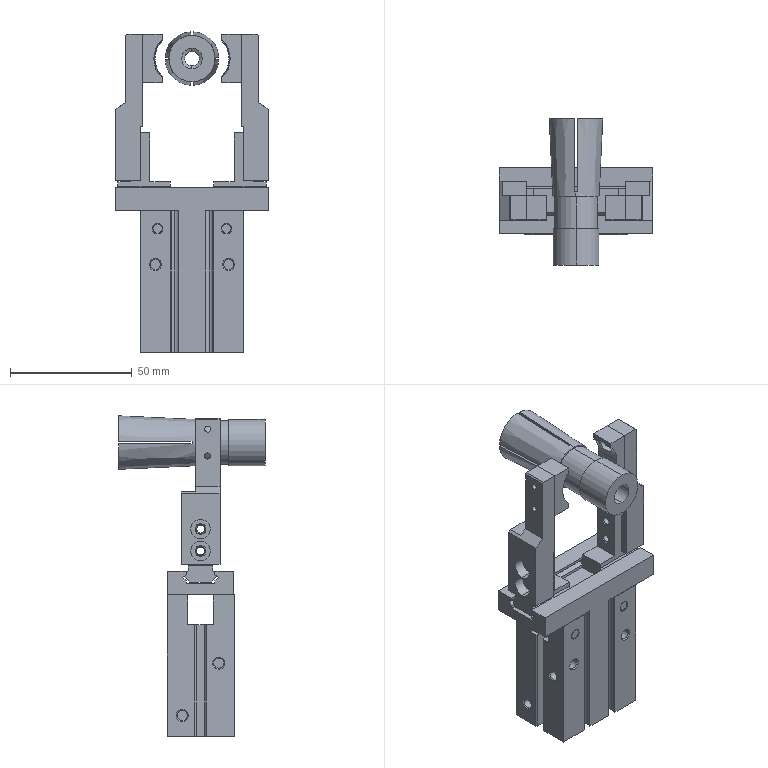Part | SolidWorks | features ReferencePattern 2, MirrorCompFeat 1 | 8 solids | 344 faces | box 63 x 60 x 131.489 mm | volume 99433 mm3 | plane 188 | cylinder 104 | cone 52 | commonest cylinder face diameters 4.134 x20 6 x10 2.5 x8 3.242 x8 3.4 x8 3.8 x8